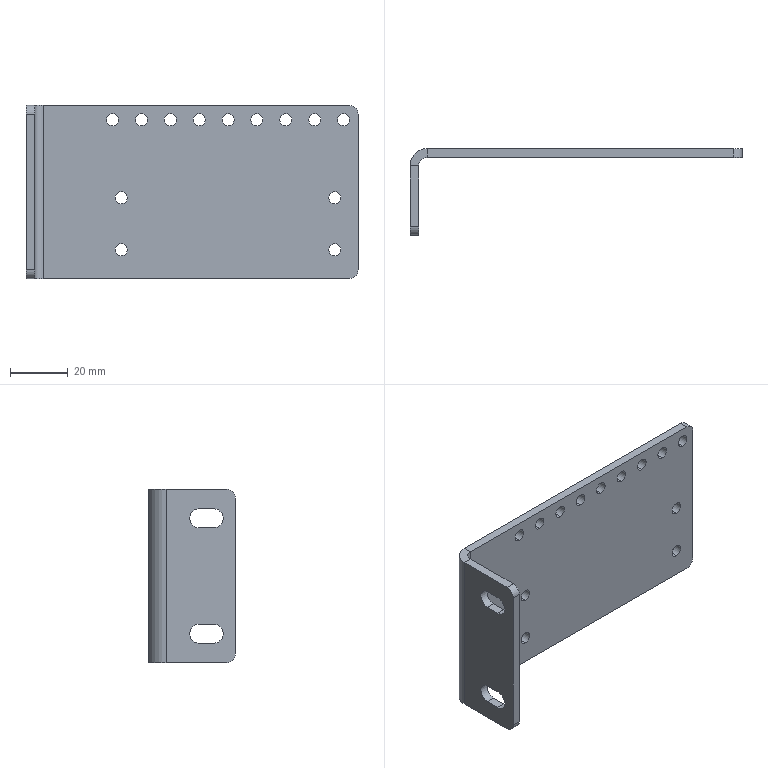Part | SolidWorks | features HoleWzd 3, Fillet 1, FlatPattern 1, SMBaseFlange 1, SheetMetal 1 | 1 solid | 52 faces | box 115 x 30 x 60 mm | volume 24246 mm3 | cylinder 36 | plane 16 | commonest cylinder face diameters 4.2 x26 6 x5 6.6 x4 12 x1